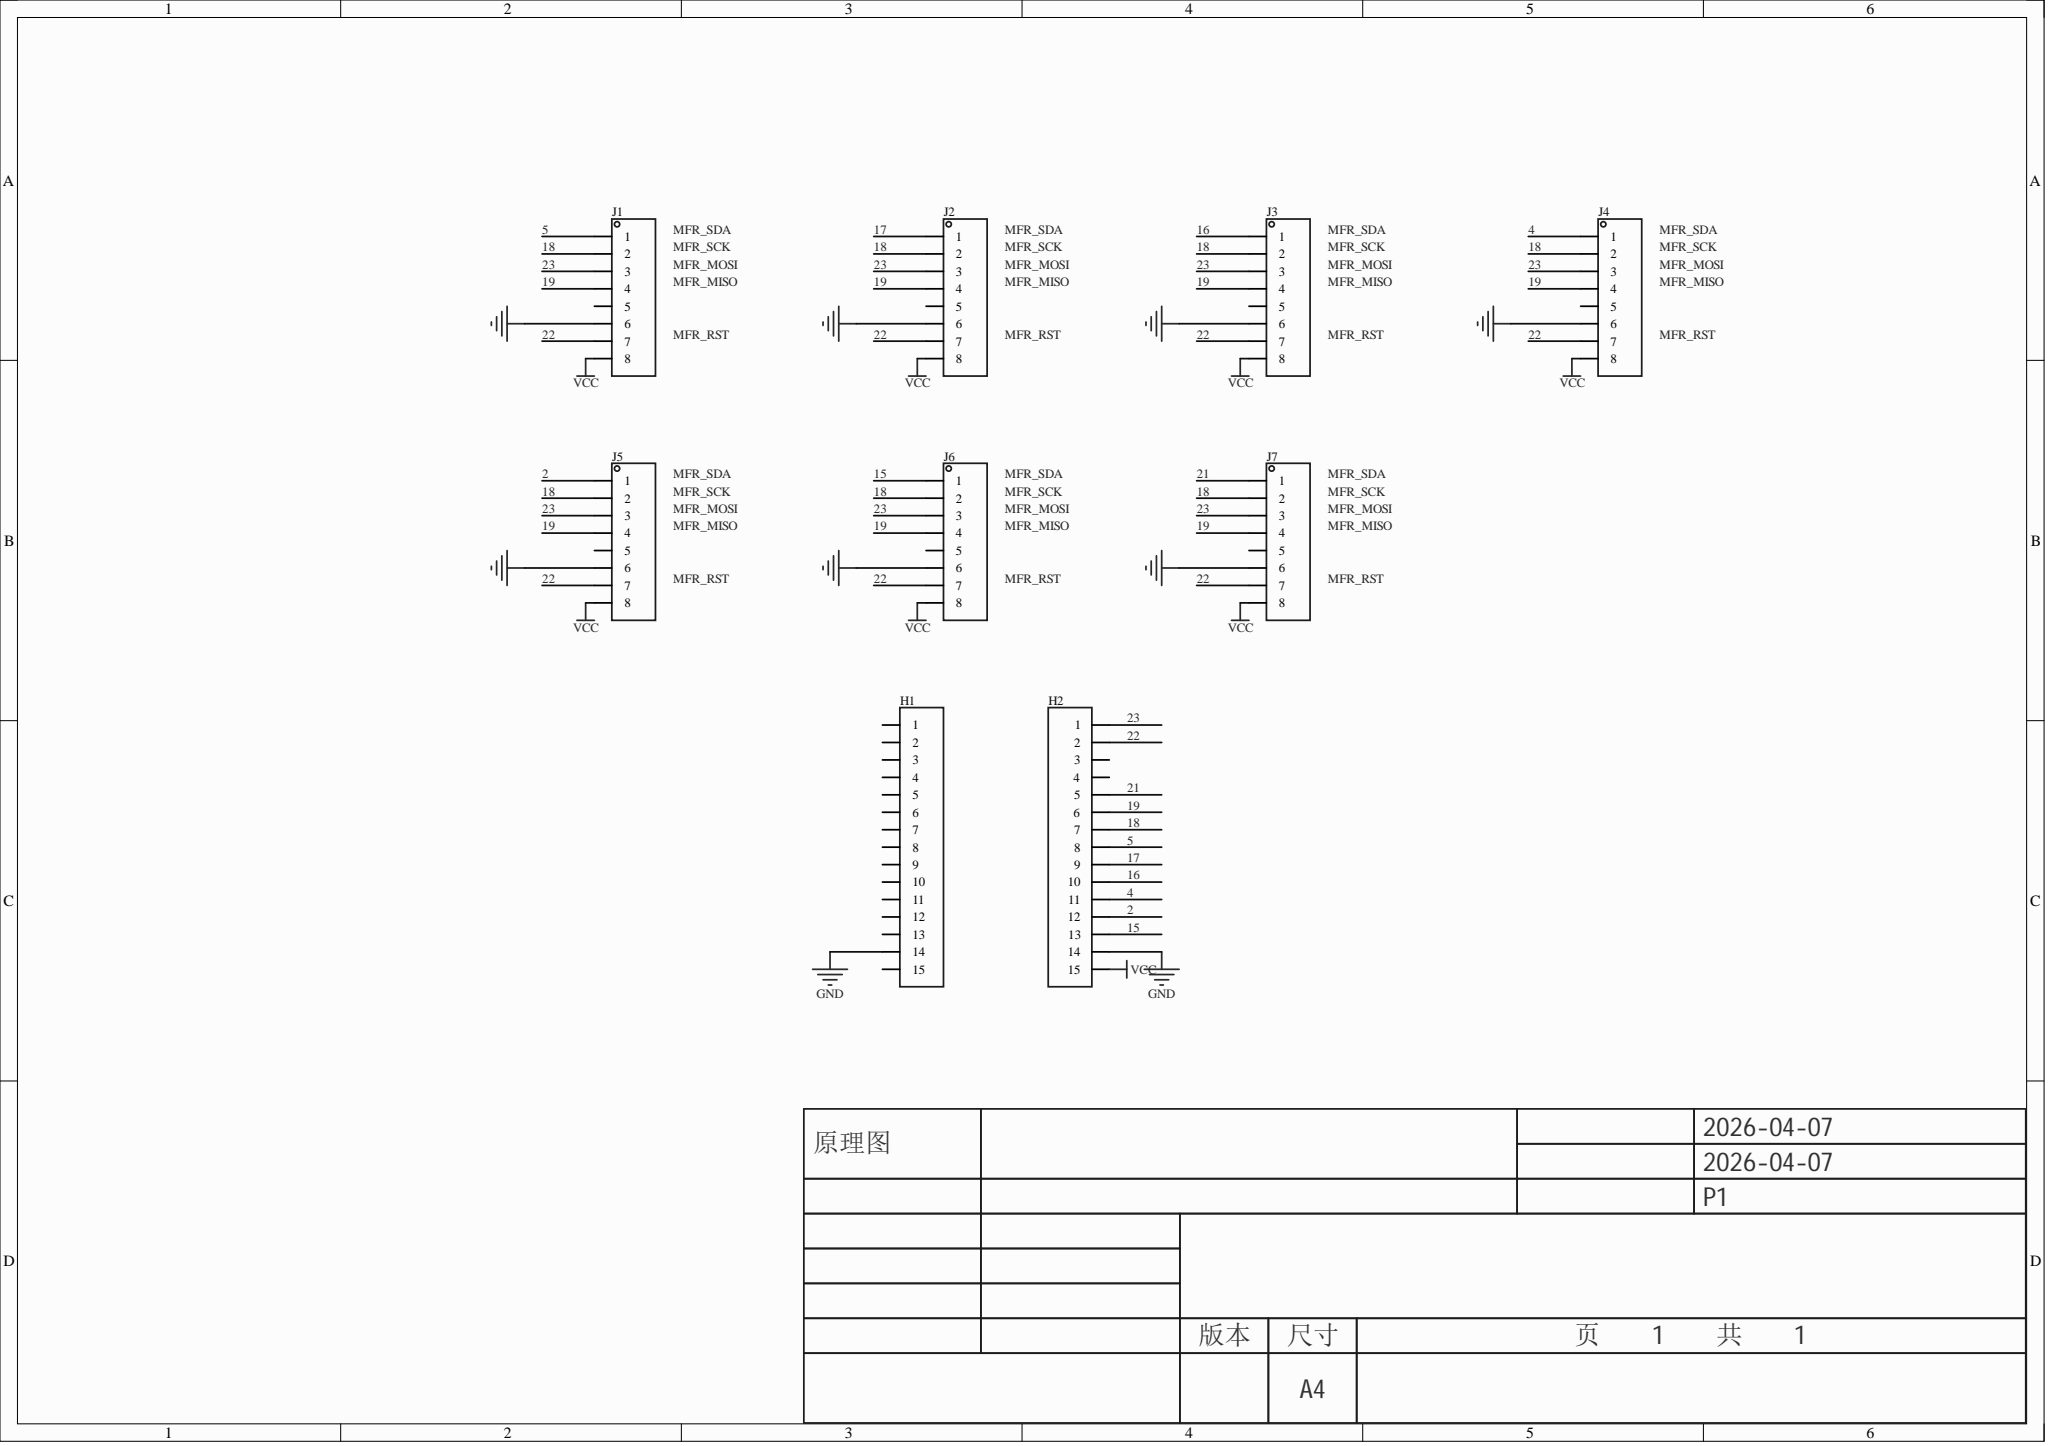Circuit board | Altium Designer | 9 parts | 13 nets
Bill of materials:
Comment,Description,Designator,Footprint,LibRef,Quantity
"","","H1, H2","HDR-TH_15P-P2.54-V-F-1","HDR-F_2.54_1x15P","2"
"","","J1, J2, J3, J4, J5, J6, J7","HDR-TH_8P-P2.54-V-M","HDR-M_2.54_1x8P","7"
Netlist (Protel format):
[
H1
HDR-TH_15P-P2.54-V-F-1




]
[
H2
HDR-TH_15P-P2.54-V-F-1




]
[
J1
HDR-TH_8P-P2.54-V-M




]
[
J2
HDR-TH_8P-P2.54-V-M




]
[
J3
HDR-TH_8P-P2.54-V-M




]
[
J4
HDR-TH_8P-P2.54-V-M




]
[
J5
HDR-TH_8P-P2.54-V-M




]
[
J6
HDR-TH_8P-P2.54-V-M




]
[
J7
HDR-TH_8P-P2.54-V-M




]
(
VCC
H2-15
J1-8
J2-8
J3-8
J4-8
J5-8
J6-8
J7-8
)
(
GND
H1-14
H2-14
J1-6
J2-6
J3-6
J4-6
J5-6
J6-6
J7-6
)
(
23
H2-1
J1-3
J2-3
J3-3
J4-3
J5-3
J6-3
J7-3
)
(
22
H2-2
J1-7
J2-7
J3-7
J4-7
J5-7
J6-7
J7-7
)
(
21
H2-5
J7-1
)
(
19
H2-6
J1-4
J2-4
J3-4
J4-4
J5-4
J6-4
J7-4
)
(
18
H2-7
J1-2
J2-2
J3-2
J4-2
J5-2
J6-2
J7-2
)
(
17
H2-9
J2-1
)
(
16
H2-10
J3-1
)
(
15
H2-13
J6-1
)
(
5
H2-8
J1-1
)
(
4
H2-11
J4-1
)
(
2
H2-12
J5-1
)